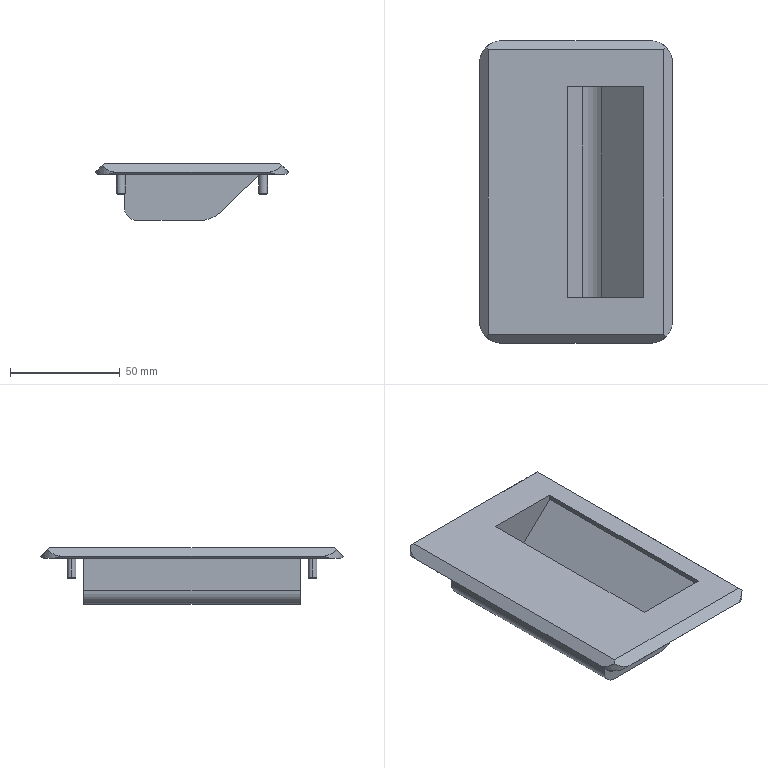Part | SolidWorks | features BaseBody 1 | 1 solid | 48 faces | box 88 x 138 x 26 mm | volume 105651 mm3 | plane 25 | cylinder 15 | cone 8 | commonest cylinder face diameters 4 x8 20 x4 24.8 x2 12.4 x1
STEP:
#1=CARTESIAN_POINT('',(34.5,55.,-8.621));
#2=VERTEX_POINT('',#1);
#3=CARTESIAN_POINT('',(30.5,55.,-8.621));
#4=VERTEX_POINT('',#3);
#5=CARTESIAN_POINT('',(32.5,55.,-8.621));
#6=DIRECTION('',(0.,0.,1.));
#7=DIRECTION('',(1.,0.,0.));
#8=AXIS2_PLACEMENT_3D('',#5,#6,#7);
#9=CIRCLE('',#8,2.);
#10=EDGE_CURVE('',#2,#4,#9,.T.);
#11=ORIENTED_EDGE('',*,*,#10,.T.);
#12=CARTESIAN_POINT('',(30.5,55.,0.));
#13=VERTEX_POINT('',#12);
#14=CARTESIAN_POINT('',(30.5,55.,-4.311));
#15=DIRECTION('',(0.,0.,1.));
#16=VECTOR('',#15,1000.);
#17=LINE('',#14,#16);
#18=EDGE_CURVE('',#4,#13,#17,.T.);
#19=ORIENTED_EDGE('',*,*,#18,.T.);
#20=CARTESIAN_POINT('',(34.5,55.,0.));
#21=VERTEX_POINT('',#20);
#22=CARTESIAN_POINT('',(32.5,55.,0.));
#23=DIRECTION('',(0.,0.,-1.));
#24=DIRECTION('',(1.,0.,0.));
#25=AXIS2_PLACEMENT_3D('',#22,#23,#24);
#26=CIRCLE('',#25,2.);
#27=EDGE_CURVE('',#13,#21,#26,.T.);
#28=ORIENTED_EDGE('',*,*,#27,.T.);
#29=CARTESIAN_POINT('',(34.5,55.,-4.311));
#30=DIRECTION('',(0.,0.,1.));
#31=VECTOR('',#30,1000.);
#32=LINE('',#29,#31);
#33=EDGE_CURVE('',#2,#21,#32,.T.);
#34=ORIENTED_EDGE('',*,*,#33,.F.);
#35=EDGE_LOOP('',(#11,#19,#28,#34));
#36=FACE_OUTER_BOUND('',#35,.T.);
#37=CARTESIAN_POINT('',(32.5,55.,-4.311));
#38=DIRECTION('',(0.,0.,1.));
#39=DIRECTION('',(1.,0.,0.));
#40=AXIS2_PLACEMENT_3D('',#37,#38,#39);
#41=CYLINDRICAL_SURFACE('',#40,2.);
#42=ADVANCED_FACE('',(#36),#41,.T.);
#43=CARTESIAN_POINT('',(34.5,-55.,-8.621));
#44=VERTEX_POINT('',#43);
#45=CARTESIAN_POINT('',(30.5,-55.,-8.621));
#46=VERTEX_POINT('',#45);
#47=CARTESIAN_POINT('',(32.5,-55.,-8.621));
#48=DIRECTION('',(0.,0.,1.));
#49=DIRECTION('',(1.,0.,0.));
#50=AXIS2_PLACEMENT_3D('',#47,#48,#49);
#51=CIRCLE('',#50,2.);
#52=EDGE_CURVE('',#44,#46,#51,.T.);
#53=ORIENTED_EDGE('',*,*,#52,.T.);
#54=CARTESIAN_POINT('',(30.5,-55.,0.));
#55=VERTEX_POINT('',#54);
#56=CARTESIAN_POINT('',(30.5,-55.,-4.311));
#57=DIRECTION('',(0.,0.,1.));
#58=VECTOR('',#57,1000.);
#59=LINE('',#56,#58);
#60=EDGE_CURVE('',#46,#55,#59,.T.);
#61=ORIENTED_EDGE('',*,*,#60,.T.);
#62=CARTESIAN_POINT('',(34.5,-55.,0.));
#63=VERTEX_POINT('',#62);
#64=CARTESIAN_POINT('',(32.5,-55.,0.));
#65=DIRECTION('',(0.,0.,-1.));
#66=DIRECTION('',(1.,0.,0.));
#67=AXIS2_PLACEMENT_3D('',#64,#65,#66);
#68=CIRCLE('',#67,2.);
#69=EDGE_CURVE('',#55,#63,#68,.T.);
#70=ORIENTED_EDGE('',*,*,#69,.T.);
#71=CARTESIAN_POINT('',(34.5,-55.,-4.311));
#72=DIRECTION('',(0.,0.,1.));
#73=VECTOR('',#72,1000.);
#74=LINE('',#71,#73);
#75=EDGE_CURVE('',#44,#63,#74,.T.);
#76=ORIENTED_EDGE('',*,*,#75,.F.);
#77=EDGE_LOOP('',(#53,#61,#70,#76));
#78=FACE_OUTER_BOUND('',#77,.T.);
#79=CARTESIAN_POINT('',(32.5,-55.,-4.311));
#80=DIRECTION('',(0.,0.,1.));
#81=DIRECTION('',(1.,0.,0.));
#82=AXIS2_PLACEMENT_3D('',#79,#80,#81);
#83=CYLINDRICAL_SURFACE('',#82,2.);
#84=ADVANCED_FACE('',(#78),#83,.T.);
#85=CARTESIAN_POINT('',(-30.5,-55.,-8.621));
#86=VERTEX_POINT('',#85);
#87=CARTESIAN_POINT('',(-34.5,-55.,-8.621));
#88=VERTEX_POINT('',#87);
#89=CARTESIAN_POINT('',(-32.5,-55.,-8.621));
#90=DIRECTION('',(0.,0.,1.));
#91=DIRECTION('',(1.,0.,0.));
#92=AXIS2_PLACEMENT_3D('',#89,#90,#91);
#93=CIRCLE('',#92,2.);
#94=EDGE_CURVE('',#86,#88,#93,.T.);
#95=ORIENTED_EDGE('',*,*,#94,.T.);
#96=CARTESIAN_POINT('',(-34.5,-55.,0.));
#97=VERTEX_POINT('',#96);
#98=CARTESIAN_POINT('',(-34.5,-55.,-4.311));
#99=DIRECTION('',(0.,0.,1.));
#100=VECTOR('',#99,1000.);
#101=LINE('',#98,#100);
#102=EDGE_CURVE('',#88,#97,#101,.T.);
#103=ORIENTED_EDGE('',*,*,#102,.T.);
#104=CARTESIAN_POINT('',(-30.5,-55.,0.));
#105=VERTEX_POINT('',#104);
#106=CARTESIAN_POINT('',(-32.5,-55.,0.));
#107=DIRECTION('',(0.,0.,-1.));
#108=DIRECTION('',(1.,0.,0.));
#109=AXIS2_PLACEMENT_3D('',#106,#107,#108);
#110=CIRCLE('',#109,2.);
#111=EDGE_CURVE('',#97,#105,#110,.T.);
#112=ORIENTED_EDGE('',*,*,#111,.T.);
#113=CARTESIAN_POINT('',(-30.5,-55.,-4.311));
#114=DIRECTION('',(0.,0.,1.));
#115=VECTOR('',#114,1000.);
#116=LINE('',#113,#115);
#117=EDGE_CURVE('',#86,#105,#116,.T.);
#118=ORIENTED_EDGE('',*,*,#117,.F.);
#119=EDGE_LOOP('',(#95,#103,#112,#118));
#120=FACE_OUTER_BOUND('',#119,.T.);
#121=CARTESIAN_POINT('',(-32.5,-55.,-4.311));
#122=DIRECTION('',(0.,0.,1.));
#123=DIRECTION('',(1.,0.,0.));
#124=AXIS2_PLACEMENT_3D('',#121,#122,#123);
#125=CYLINDRICAL_SURFACE('',#124,2.);
#126=ADVANCED_FACE('',(#120),#125,.T.);
#127=CARTESIAN_POINT('',(-30.5,55.,-8.621));
#128=VERTEX_POINT('',#127);
#129=CARTESIAN_POINT('',(-34.5,55.,-8.621));
#130=VERTEX_POINT('',#129);
#131=CARTESIAN_POINT('',(-32.5,55.,-8.621));
#132=DIRECTION('',(0.,0.,1.));
#133=DIRECTION('',(1.,0.,0.));
#134=AXIS2_PLACEMENT_3D('',#131,#132,#133);
#135=CIRCLE('',#134,2.);
#136=EDGE_CURVE('',#128,#130,#135,.T.);
#137=ORIENTED_EDGE('',*,*,#136,.T.);
#138=CARTESIAN_POINT('',(-34.5,55.,0.));
#139=VERTEX_POINT('',#138);
#140=CARTESIAN_POINT('',(-34.5,55.,-4.311));
#141=DIRECTION('',(0.,0.,1.));
#142=VECTOR('',#141,1000.);
#143=LINE('',#140,#142);
#144=EDGE_CURVE('',#130,#139,#143,.T.);
#145=ORIENTED_EDGE('',*,*,#144,.T.);
#146=CARTESIAN_POINT('',(-30.5,55.,0.));
#147=VERTEX_POINT('',#146);
#148=CARTESIAN_POINT('',(-32.5,55.,0.));
#149=DIRECTION('',(0.,0.,-1.));
#150=DIRECTION('',(1.,0.,0.));
#151=AXIS2_PLACEMENT_3D('',#148,#149,#150);
#152=CIRCLE('',#151,2.);
#153=EDGE_CURVE('',#139,#147,#152,.T.);
#154=ORIENTED_EDGE('',*,*,#153,.T.);
#155=CARTESIAN_POINT('',(-30.5,55.,-4.311));
#156=DIRECTION('',(0.,0.,1.));
#157=VECTOR('',#156,1000.);
#158=LINE('',#155,#157);
#159=EDGE_CURVE('',#128,#147,#158,.T.);
#160=ORIENTED_EDGE('',*,*,#159,.F.);
#161=EDGE_LOOP('',(#137,#145,#154,#160));
#162=FACE_OUTER_BOUND('',#161,.T.);
#163=CARTESIAN_POINT('',(-32.5,55.,-4.311));
#164=DIRECTION('',(0.,0.,1.));
#165=DIRECTION('',(1.,0.,0.));
#166=AXIS2_PLACEMENT_3D('',#163,#164,#165);
#167=CYLINDRICAL_SURFACE('',#166,2.);
#168=ADVANCED_FACE('',(#162),#167,.T.);
#169=CARTESIAN_POINT('',(34.121,55.,-9.));
#170=VERTEX_POINT('',#169);
#171=CARTESIAN_POINT('',(30.879,55.,-9.));
#172=VERTEX_POINT('',#171);
#173=CARTESIAN_POINT('',(32.5,55.,-9.));
#174=DIRECTION('',(0.,0.,1.));
#175=DIRECTION('',(1.,0.,0.));
#176=AXIS2_PLACEMENT_3D('',#173,#174,#175);
#177=CIRCLE('',#176,1.621);
#178=EDGE_CURVE('',#170,#172,#177,.T.);
#179=ORIENTED_EDGE('',*,*,#178,.T.);
#180=CARTESIAN_POINT('',(30.5,55.,-8.621));
#181=DIRECTION('',(-0.7071,0.,0.7071));
#182=VECTOR('',#181,1000.);
#183=LINE('',#180,#182);
#184=EDGE_CURVE('',#172,#4,#183,.T.);
#185=ORIENTED_EDGE('',*,*,#184,.T.);
#186=ORIENTED_EDGE('',*,*,#10,.F.);
#187=CARTESIAN_POINT('',(34.5,55.,-8.621));
#188=DIRECTION('',(0.7071,0.,0.7071));
#189=VECTOR('',#188,1000.);
#190=LINE('',#187,#189);
#191=EDGE_CURVE('',#170,#2,#190,.T.);
#192=ORIENTED_EDGE('',*,*,#191,.F.);
#193=EDGE_LOOP('',(#179,#185,#186,#192));
#194=FACE_OUTER_BOUND('',#193,.T.);
#195=CARTESIAN_POINT('',(32.5,55.,-8.621));
#196=DIRECTION('',(0.,0.,1.));
#197=DIRECTION('',(1.,0.,0.));
#198=AXIS2_PLACEMENT_3D('',#195,#196,#197);
#199=CONICAL_SURFACE('',#198,2.,0.7854);
#200=ADVANCED_FACE('',(#194),#199,.T.);
#201=CARTESIAN_POINT('',(34.121,-55.,-9.));
#202=VERTEX_POINT('',#201);
#203=CARTESIAN_POINT('',(30.879,-55.,-9.));
#204=VERTEX_POINT('',#203);
#205=CARTESIAN_POINT('',(32.5,-55.,-9.));
#206=DIRECTION('',(0.,0.,1.));
#207=DIRECTION('',(1.,0.,0.));
#208=AXIS2_PLACEMENT_3D('',#205,#206,#207);
#209=CIRCLE('',#208,1.621);
#210=EDGE_CURVE('',#202,#204,#209,.T.);
#211=ORIENTED_EDGE('',*,*,#210,.T.);
#212=CARTESIAN_POINT('',(30.5,-55.,-8.621));
#213=DIRECTION('',(-0.7071,0.,0.7071));
#214=VECTOR('',#213,1000.);
#215=LINE('',#212,#214);
#216=EDGE_CURVE('',#204,#46,#215,.T.);
#217=ORIENTED_EDGE('',*,*,#216,.T.);
#218=ORIENTED_EDGE('',*,*,#52,.F.);
#219=CARTESIAN_POINT('',(34.5,-55.,-8.621));
#220=DIRECTION('',(0.7071,0.,0.7071));
#221=VECTOR('',#220,1000.);
#222=LINE('',#219,#221);
#223=EDGE_CURVE('',#202,#44,#222,.T.);
#224=ORIENTED_EDGE('',*,*,#223,.F.);
#225=EDGE_LOOP('',(#211,#217,#218,#224));
#226=FACE_OUTER_BOUND('',#225,.T.);
#227=CARTESIAN_POINT('',(32.5,-55.,-8.621));
#228=DIRECTION('',(0.,0.,1.));
#229=DIRECTION('',(1.,0.,0.));
#230=AXIS2_PLACEMENT_3D('',#227,#228,#229);
#231=CONICAL_SURFACE('',#230,2.,0.7854);
#232=ADVANCED_FACE('',(#226),#231,.T.);
#233=CARTESIAN_POINT('',(-30.879,-55.,-9.));
#234=VERTEX_POINT('',#233);
#235=CARTESIAN_POINT('',(-34.121,-55.,-9.));
#236=VERTEX_POINT('',#235);
#237=CARTESIAN_POINT('',(-32.5,-55.,-9.));
#238=DIRECTION('',(0.,0.,1.));
#239=DIRECTION('',(1.,0.,0.));
#240=AXIS2_PLACEMENT_3D('',#237,#238,#239);
#241=CIRCLE('',#240,1.621);
#242=EDGE_CURVE('',#234,#236,#241,.T.);
#243=ORIENTED_EDGE('',*,*,#242,.T.);
#244=CARTESIAN_POINT('',(-34.5,-55.,-8.621));
#245=DIRECTION('',(-0.7071,0.,0.7071));
#246=VECTOR('',#245,1000.);
#247=LINE('',#244,#246);
#248=EDGE_CURVE('',#236,#88,#247,.T.);
#249=ORIENTED_EDGE('',*,*,#248,.T.);
#250=ORIENTED_EDGE('',*,*,#94,.F.);
#251=CARTESIAN_POINT('',(-30.5,-55.,-8.621));
#252=DIRECTION('',(0.7071,0.,0.7071));
#253=VECTOR('',#252,1000.);
#254=LINE('',#251,#253);
#255=EDGE_CURVE('',#234,#86,#254,.T.);
#256=ORIENTED_EDGE('',*,*,#255,.F.);
#257=EDGE_LOOP('',(#243,#249,#250,#256));
#258=FACE_OUTER_BOUND('',#257,.T.);
#259=CARTESIAN_POINT('',(-32.5,-55.,-8.621));
#260=DIRECTION('',(0.,0.,1.));
#261=DIRECTION('',(1.,0.,0.));
#262=AXIS2_PLACEMENT_3D('',#259,#260,#261);
#263=CONICAL_SURFACE('',#262,2.,0.7854);
#264=ADVANCED_FACE('',(#258),#263,.T.);
#265=CARTESIAN_POINT('',(-30.879,55.,-9.));
#266=VERTEX_POINT('',#265);
#267=CARTESIAN_POINT('',(-34.121,55.,-9.));
#268=VERTEX_POINT('',#267);
#269=CARTESIAN_POINT('',(-32.5,55.,-9.));
#270=DIRECTION('',(0.,0.,1.));
#271=DIRECTION('',(1.,0.,0.));
#272=AXIS2_PLACEMENT_3D('',#269,#270,#271);
#273=CIRCLE('',#272,1.621);
#274=EDGE_CURVE('',#266,#268,#273,.T.);
#275=ORIENTED_EDGE('',*,*,#274,.T.);
#276=CARTESIAN_POINT('',(-34.5,55.,-8.621));
#277=DIRECTION('',(-0.7071,0.,0.7071));
#278=VECTOR('',#277,1000.);
#279=LINE('',#276,#278);
#280=EDGE_CURVE('',#268,#130,#279,.T.);
#281=ORIENTED_EDGE('',*,*,#280,.T.);
#282=ORIENTED_EDGE('',*,*,#136,.F.);
#283=CARTESIAN_POINT('',(-30.5,55.,-8.621));
#284=DIRECTION('',(0.7071,0.,0.7071));
#285=VECTOR('',#284,1000.);
#286=LINE('',#283,#285);
#287=EDGE_CURVE('',#266,#128,#286,.T.);
#288=ORIENTED_EDGE('',*,*,#287,.F.);
#289=EDGE_LOOP('',(#275,#281,#282,#288));
#290=FACE_OUTER_BOUND('',#289,.T.);
#291=CARTESIAN_POINT('',(-32.5,55.,-8.621));
#292=DIRECTION('',(0.,0.,1.));
#293=DIRECTION('',(1.,0.,0.));
#294=AXIS2_PLACEMENT_3D('',#291,#292,#293);
#295=CONICAL_SURFACE('',#294,2.,0.7854);
#296=ADVANCED_FACE('',(#290),#295,.T.);
#297=ORIENTED_EDGE('',*,*,#274,.F.);
#298=CARTESIAN_POINT('',(-32.5,55.,-9.));
#299=DIRECTION('',(0.,0.,1.));
#300=DIRECTION('',(1.,0.,0.));
#301=AXIS2_PLACEMENT_3D('',#298,#299,#300);
#302=CIRCLE('',#301,1.621);
#303=EDGE_CURVE('',#268,#266,#302,.T.);
#304=ORIENTED_EDGE('',*,*,#303,.F.);
#305=EDGE_LOOP('',(#297,#304));
#306=FACE_OUTER_BOUND('',#305,.T.);
#307=CARTESIAN_POINT('',(-31.69,55.,-9.));
#308=DIRECTION('',(0.,0.,-1.));
#309=DIRECTION('',(0.,-1.,0.));
#310=AXIS2_PLACEMENT_3D('',#307,#308,#309);
#311=PLANE('',#310);
#312=ADVANCED_FACE('',(#306),#311,.T.);
#313=ORIENTED_EDGE('',*,*,#242,.F.);
#314=CARTESIAN_POINT('',(-32.5,-55.,-9.));
#315=DIRECTION('',(0.,0.,1.));
#316=DIRECTION('',(1.,0.,0.));
#317=AXIS2_PLACEMENT_3D('',#314,#315,#316);
#318=CIRCLE('',#317,1.621);
#319=EDGE_CURVE('',#236,#234,#318,.T.);
#320=ORIENTED_EDGE('',*,*,#319,.F.);
#321=EDGE_LOOP('',(#313,#320));
#322=FACE_OUTER_BOUND('',#321,.T.);
#323=CARTESIAN_POINT('',(-31.69,-55.,-9.));
#324=DIRECTION('',(0.,0.,-1.));
#325=DIRECTION('',(0.,-1.,0.));
#326=AXIS2_PLACEMENT_3D('',#323,#324,#325);
#327=PLANE('',#326);
#328=ADVANCED_FACE('',(#322),#327,.T.);
#329=ORIENTED_EDGE('',*,*,#210,.F.);
#330=CARTESIAN_POINT('',(32.5,-55.,-9.));
#331=DIRECTION('',(0.,0.,1.));
#332=DIRECTION('',(1.,0.,0.));
#333=AXIS2_PLACEMENT_3D('',#330,#331,#332);
#334=CIRCLE('',#333,1.621);
#335=EDGE_CURVE('',#204,#202,#334,.T.);
#336=ORIENTED_EDGE('',*,*,#335,.F.);
#337=EDGE_LOOP('',(#329,#336));
#338=FACE_OUTER_BOUND('',#337,.T.);
#339=CARTESIAN_POINT('',(33.31,-55.,-9.));
#340=DIRECTION('',(0.,0.,-1.));
#341=DIRECTION('',(0.,-1.,0.));
#342=AXIS2_PLACEMENT_3D('',#339,#340,#341);
#343=PLANE('',#342);
#344=ADVANCED_FACE('',(#338),#343,.T.);
#345=ORIENTED_EDGE('',*,*,#178,.F.);
#346=CARTESIAN_POINT('',(32.5,55.,-9.));
#347=DIRECTION('',(0.,0.,1.));
#348=DIRECTION('',(1.,0.,0.));
#349=AXIS2_PLACEMENT_3D('',#346,#347,#348);
#350=CIRCLE('',#349,1.621);
#351=EDGE_CURVE('',#172,#170,#350,.T.);
#352=ORIENTED_EDGE('',*,*,#351,.F.);
#353=EDGE_LOOP('',(#345,#352));
#354=FACE_OUTER_BOUND('',#353,.T.);
#355=CARTESIAN_POINT('',(33.31,55.,-9.));
#356=DIRECTION('',(0.,0.,-1.));
#357=DIRECTION('',(0.,-1.,0.));
#358=AXIS2_PLACEMENT_3D('',#355,#356,#357);
#359=PLANE('',#358);
#360=ADVANCED_FACE('',(#354),#359,.T.);
#361=CARTESIAN_POINT('',(12.445,49.5,-17.597));
#362=VERTEX_POINT('',#361);
#363=CARTESIAN_POINT('',(3.912,49.5,-21.));
#364=VERTEX_POINT('',#363);
#365=CARTESIAN_POINT('',(3.912,49.5,-8.6));
#366=DIRECTION('',(0.,1.,0.));
#367=DIRECTION('',(0.,0.,1.));
#368=AXIS2_PLACEMENT_3D('',#365,#366,#367);
#369=CIRCLE('',#368,12.4);
#370=EDGE_CURVE('',#362,#364,#369,.T.);
#371=ORIENTED_EDGE('',*,*,#370,.F.);
#372=CARTESIAN_POINT('',(12.445,-49.5,-17.597));
#373=VERTEX_POINT('',#372);
#374=CARTESIAN_POINT('',(12.445,49.5,-17.597));
#375=DIRECTION('',(0.,1.,0.));
#376=VECTOR('',#375,1000.);
#377=LINE('',#374,#376);
#378=EDGE_CURVE('',#373,#362,#377,.T.);
#379=ORIENTED_EDGE('',*,*,#378,.F.);
#380=CARTESIAN_POINT('',(3.912,-49.5,-21.));
#381=VERTEX_POINT('',#380);
#382=CARTESIAN_POINT('',(3.912,-49.5,-8.6));
#383=DIRECTION('',(0.,1.,0.));
#384=DIRECTION('',(0.,0.,1.));
#385=AXIS2_PLACEMENT_3D('',#382,#383,#384);
#386=CIRCLE('',#385,12.4);
#387=EDGE_CURVE('',#373,#381,#386,.T.);
#388=ORIENTED_EDGE('',*,*,#387,.T.);
#389=CARTESIAN_POINT('',(3.912,49.5,-21.));
#390=DIRECTION('',(0.,-1.,0.));
#391=VECTOR('',#390,1000.);
#392=LINE('',#389,#391);
#393=EDGE_CURVE('',#364,#381,#392,.T.);
#394=ORIENTED_EDGE('',*,*,#393,.F.);
#395=EDGE_LOOP('',(#371,#379,#388,#394));
#396=FACE_OUTER_BOUND('',#395,.T.);
#397=CARTESIAN_POINT('',(3.912,49.5,-8.6));
#398=DIRECTION('',(0.,1.,0.));
#399=DIRECTION('',(0.,0.,1.));
#400=AXIS2_PLACEMENT_3D('',#397,#398,#399);
#401=CYLINDRICAL_SURFACE('',#400,12.4);
#402=ADVANCED_FACE('',(#396),#401,.T.);
#403=CARTESIAN_POINT('',(-24.8,49.5,-21.));
#404=VERTEX_POINT('',#403);
#405=CARTESIAN_POINT('',(0.,49.5,-21.));
#406=DIRECTION('',(-1.,0.,0.));
#407=VECTOR('',#406,1000.);
#408=LINE('',#405,#407);
#409=EDGE_CURVE('',#364,#404,#408,.T.);
#410=ORIENTED_EDGE('',*,*,#409,.F.);
#411=ORIENTED_EDGE('',*,*,#393,.T.);
#412=CARTESIAN_POINT('',(-24.8,-49.5,-21.));
#413=VERTEX_POINT('',#412);
#414=CARTESIAN_POINT('',(0.,-49.5,-21.));
#415=DIRECTION('',(-1.,0.,0.));
#416=VECTOR('',#415,1000.);
#417=LINE('',#414,#416);
#418=EDGE_CURVE('',#381,#413,#417,.T.);
#419=ORIENTED_EDGE('',*,*,#418,.T.);
#420=CARTESIAN_POINT('',(-24.8,49.5,-21.));
#421=DIRECTION('',(0.,-1.,0.));
#422=VECTOR('',#421,1000.);
#423=LINE('',#420,#422);
#424=EDGE_CURVE('',#404,#413,#423,.T.);
#425=ORIENTED_EDGE('',*,*,#424,.F.);
#426=EDGE_LOOP('',(#410,#411,#419,#425));
#427=FACE_OUTER_BOUND('',#426,.T.);
#428=CARTESIAN_POINT('',(3.912,49.5,-21.));
#429=DIRECTION('',(0.,0.,-1.));
#430=DIRECTION('',(0.,-1.,0.));
#431=AXIS2_PLACEMENT_3D('',#428,#429,#430);
#432=PLANE('',#431);
#433=ADVANCED_FACE('',(#427),#432,.T.);
#434=CARTESIAN_POINT('',(-31.,49.5,-14.8));
#435=VERTEX_POINT('',#434);
#436=CARTESIAN_POINT('',(-24.8,49.5,-14.8));
#437=DIRECTION('',(0.,1.,0.));
#438=DIRECTION('',(0.,0.,1.));
#439=AXIS2_PLACEMENT_3D('',#436,#437,#438);
#440=CIRCLE('',#439,6.2);
#441=EDGE_CURVE('',#404,#435,#440,.T.);
#442=ORIENTED_EDGE('',*,*,#441,.F.);
#443=ORIENTED_EDGE('',*,*,#424,.T.);
#444=CARTESIAN_POINT('',(-31.,-49.5,-14.8));
#445=VERTEX_POINT('',#444);
#446=CARTESIAN_POINT('',(-24.8,-49.5,-14.8));
#447=DIRECTION('',(0.,1.,0.));
#448=DIRECTION('',(0.,0.,1.));
#449=AXIS2_PLACEMENT_3D('',#446,#447,#448);
#450=CIRCLE('',#449,6.2);
#451=EDGE_CURVE('',#413,#445,#450,.T.);
#452=ORIENTED_EDGE('',*,*,#451,.T.);
#453=CARTESIAN_POINT('',(-31.,49.5,-14.8));
#454=DIRECTION('',(0.,-1.,0.));
#455=VECTOR('',#454,1000.);
#456=LINE('',#453,#455);
#457=EDGE_CURVE('',#435,#445,#456,.T.);
#458=ORIENTED_EDGE('',*,*,#457,.F.);
#459=EDGE_LOOP('',(#442,#443,#452,#458));
#460=FACE_OUTER_BOUND('',#459,.T.);
#461=CARTESIAN_POINT('',(-24.8,49.5,-14.8));
#462=DIRECTION('',(0.,1.,0.));
#463=DIRECTION('',(0.,0.,1.));
#464=AXIS2_PLACEMENT_3D('',#461,#462,#463);
#465=CYLINDRICAL_SURFACE('',#464,6.2);
#466=ADVANCED_FACE('',(#460),#465,.T.);
#467=ORIENTED_EDGE('',*,*,#409,.T.);
#468=ORIENTED_EDGE('',*,*,#441,.T.);
#469=CARTESIAN_POINT('',(-31.,49.5,0.));
#470=VERTEX_POINT('',#469);
#471=CARTESIAN_POINT('',(-31.,49.5,-14.8));
#472=DIRECTION('',(0.,0.,-1.));
#473=VECTOR('',#472,1000.);
#474=LINE('',#471,#473);
#475=EDGE_CURVE('',#470,#435,#474,.T.);
#476=ORIENTED_EDGE('',*,*,#475,.F.);
#477=CARTESIAN_POINT('',(31.,49.5,0.));
#478=VERTEX_POINT('',#477);
#479=CARTESIAN_POINT('',(0.,49.5,0.));
#480=DIRECTION('',(1.,0.,0.));
#481=VECTOR('',#480,1000.);
#482=LINE('',#479,#481);
#483=EDGE_CURVE('',#470,#478,#482,.T.);
#484=ORIENTED_EDGE('',*,*,#483,.T.);
#485=CARTESIAN_POINT('',(31.,49.5,0.));
#486=DIRECTION('',(0.7256,0.,0.6881));
#487=VECTOR('',#486,1000.);
#488=LINE('',#485,#487);
#489=EDGE_CURVE('',#362,#478,#488,.T.);
#490=ORIENTED_EDGE('',*,*,#489,.F.);
#491=ORIENTED_EDGE('',*,*,#370,.T.);
#492=EDGE_LOOP('',(#467,#468,#476,#484,#490,#491));
#493=FACE_OUTER_BOUND('',#492,.T.);
#494=CARTESIAN_POINT('',(0.,49.5,0.));
#495=DIRECTION('',(0.,1.,0.));
#496=DIRECTION('',(1.,0.,0.));
#497=AXIS2_PLACEMENT_3D('',#494,#495,#496);
#498=PLANE('',#497);
#499=ADVANCED_FACE('',(#493),#498,.T.);
#500=ORIENTED_EDGE('',*,*,#489,.T.);
#501=CARTESIAN_POINT('',(31.,-49.5,0.));
#502=VERTEX_POINT('',#501);
#503=CARTESIAN_POINT('',(31.,0.,0.));
#504=DIRECTION('',(0.,-1.,0.));
#505=VECTOR('',#504,1000.);
#506=LINE('',#503,#505);
#507=EDGE_CURVE('',#478,#502,#506,.T.);
#508=ORIENTED_EDGE('',*,*,#507,.T.);
#509=CARTESIAN_POINT('',(31.,-49.5,0.));
#510=DIRECTION('',(-0.7256,0.,-0.6881));
#511=VECTOR('',#510,1000.);
#512=LINE('',#509,#511);
#513=EDGE_CURVE('',#502,#373,#512,.T.);
#514=ORIENTED_EDGE('',*,*,#513,.T.);
#515=ORIENTED_EDGE('',*,*,#378,.T.);
#516=EDGE_LOOP('',(#500,#508,#514,#515));
#517=FACE_OUTER_BOUND('',#516,.T.);
#518=CARTESIAN_POINT('',(31.,49.5,0.));
#519=DIRECTION('',(0.6881,0.,-0.7256));
#520=DIRECTION('',(0.,-1.,0.));
#521=AXIS2_PLACEMENT_3D('',#518,#519,#520);
#522=PLANE('',#521);
#523=ADVANCED_FACE('',(#517),#522,.T.);
#524=CARTESIAN_POINT('',(-31.,-49.5,0.));
#525=VERTEX_POINT('',#524);
#526=CARTESIAN_POINT('',(-31.,-49.5,-14.8));
#527=DIRECTION('',(0.,0.,1.));
#528=VECTOR('',#527,1000.);
#529=LINE('',#526,#528);
#530=EDGE_CURVE('',#445,#525,#529,.T.);
#531=ORIENTED_EDGE('',*,*,#530,.F.);
#532=ORIENTED_EDGE('',*,*,#451,.F.);
#533=ORIENTED_EDGE('',*,*,#418,.F.);
#534=ORIENTED_EDGE('',*,*,#387,.F.);
#535=ORIENTED_EDGE('',*,*,#513,.F.);
#536=CARTESIAN_POINT('',(0.,-49.5,0.));
#537=DIRECTION('',(-1.,0.,0.));
#538=VECTOR('',#537,1000.);
#539=LINE('',#536,#538);
#540=EDGE_CURVE('',#502,#525,#539,.T.);
#541=ORIENTED_EDGE('',*,*,#540,.T.);
#542=EDGE_LOOP('',(#531,#532,#533,#534,#535,#541));
#543=FACE_OUTER_BOUND('',#542,.T.);
#544=CARTESIAN_POINT('',(0.,-49.5,0.));
#545=DIRECTION('',(0.,1.,0.));
#546=DIRECTION('',(1.,0.,0.));
#547=AXIS2_PLACEMENT_3D('',#544,#545,#546);
#548=PLANE('',#547);
#549=ADVANCED_FACE('',(#543),#548,.F.);
#550=ORIENTED_EDGE('',*,*,#475,.T.);
#551=ORIENTED_EDGE('',*,*,#457,.T.);
#552=ORIENTED_EDGE('',*,*,#530,.T.);
#553=CARTESIAN_POINT('',(-31.,0.,0.));
#554=DIRECTION('',(0.,1.,0.));
#555=VECTOR('',#554,1000.);
#556=LINE('',#553,#555);
#557=EDGE_CURVE('',#525,#470,#556,.T.);
#558=ORIENTED_EDGE('',*,*,#557,.T.);
#559=EDGE_LOOP('',(#550,#551,#552,#558));
#560=FACE_OUTER_BOUND('',#559,.T.);
#561=CARTESIAN_POINT('',(-31.,49.5,-14.8));
#562=DIRECTION('',(-1.,0.,0.));
#563=DIRECTION('',(0.,1.,0.));
#564=AXIS2_PLACEMENT_3D('',#561,#562,#563);
#565=PLANE('',#564);
#566=ADVANCED_FACE('',(#560),#565,.T.);
#567=CARTESIAN_POINT('',(-32.5,55.,0.));
#568=DIRECTION('',(0.,0.,-1.));
#569=DIRECTION('',(1.,0.,0.));
#570=AXIS2_PLACEMENT_3D('',#567,#568,#569);
#571=CIRCLE('',#570,2.);
#572=EDGE_CURVE('',#147,#139,#571,.T.);
#573=ORIENTED_EDGE('',*,*,#572,.F.);
#574=ORIENTED_EDGE('',*,*,#153,.F.);
#575=EDGE_LOOP('',(#573,#574));
#576=FACE_BOUND('',#575,.T.);
#577=CARTESIAN_POINT('',(-32.5,-55.,0.));
#578=DIRECTION('',(0.,0.,-1.));
#579=DIRECTION('',(1.,0.,0.));
#580=AXIS2_PLACEMENT_3D('',#577,#578,#579);
#581=CIRCLE('',#580,2.);
#582=EDGE_CURVE('',#105,#97,#581,.T.);
#583=ORIENTED_EDGE('',*,*,#582,.F.);
#584=ORIENTED_EDGE('',*,*,#111,.F.);
#585=EDGE_LOOP('',(#583,#584));
#586=FACE_BOUND('',#585,.T.);
#587=CARTESIAN_POINT('',(32.5,-55.,0.));
#588=DIRECTION('',(0.,0.,-1.));
#589=DIRECTION('',(1.,0.,0.));
#590=AXIS2_PLACEMENT_3D('',#587,#588,#589);
#591=CIRCLE('',#590,2.);
#592=EDGE_CURVE('',#63,#55,#591,.T.);
#593=ORIENTED_EDGE('',*,*,#592,.F.);
#594=ORIENTED_EDGE('',*,*,#69,.F.);
#595=EDGE_LOOP('',(#593,#594));
#596=FACE_BOUND('',#595,.T.);
#597=CARTESIAN_POINT('',(32.5,55.,0.));
#598=DIRECTION('',(0.,0.,-1.));
#599=DIRECTION('',(1.,0.,0.));
#600=AXIS2_PLACEMENT_3D('',#597,#598,#599);
#601=CIRCLE('',#600,2.);
#602=EDGE_CURVE('',#21,#13,#601,.T.);
#603=ORIENTED_EDGE('',*,*,#602,.F.);
#604=ORIENTED_EDGE('',*,*,#27,.F.);
#605=EDGE_LOOP('',(#603,#604));
#606=FACE_BOUND('',#605,.T.);
#607=ORIENTED_EDGE('',*,*,#540,.F.);
#608=ORIENTED_EDGE('',*,*,#507,.F.);
#609=ORIENTED_EDGE('',*,*,#483,.F.);
#610=ORIENTED_EDGE('',*,*,#557,.F.);
#611=EDGE_LOOP('',(#607,#608,#609,#610));
#612=FACE_BOUND('',#611,.T.);
#613=CARTESIAN_POINT('',(-38.359,68.,0.));
#614=VERTEX_POINT('',#613);
#615=CARTESIAN_POINT('',(-43.,63.359,0.));
#616=VERTEX_POINT('',#615);
#617=CARTESIAN_POINT('',(-34.,59.,0.));
#618=DIRECTION('',(0.,0.,1.));
#619=DIRECTION('',(-1.,0.,0.));
#620=AXIS2_PLACEMENT_3D('',#617,#618,#619);
#621=CIRCLE('',#620,10.);
#622=EDGE_CURVE('',#614,#616,#621,.T.);
#623=ORIENTED_EDGE('',*,*,#622,.F.);
#624=CARTESIAN_POINT('',(38.359,68.,0.));
#625=VERTEX_POINT('',#624);
#626=CARTESIAN_POINT('',(44.,68.,0.));
#627=DIRECTION('',(1.,0.,0.));
#628=VECTOR('',#627,1000.);
#629=LINE('',#626,#628);
#630=EDGE_CURVE('',#614,#625,#629,.T.);
#631=ORIENTED_EDGE('',*,*,#630,.T.);
#632=CARTESIAN_POINT('',(43.,63.359,0.));
#633=VERTEX_POINT('',#632);
#634=CARTESIAN_POINT('',(34.,59.,0.));
#635=DIRECTION('',(0.,0.,1.));
#636=DIRECTION('',(-1.,0.,0.));
#637=AXIS2_PLACEMENT_3D('',#634,#635,#636);
#638=CIRCLE('',#637,10.);
#639=EDGE_CURVE('',#633,#625,#638,.T.);
#640=ORIENTED_EDGE('',*,*,#639,.F.);
#641=CARTESIAN_POINT('',(43.,-63.359,0.));
#642=VERTEX_POINT('',#641);
#643=CARTESIAN_POINT('',(43.,69.,0.));
#644=DIRECTION('',(0.,-1.,0.));
#645=VECTOR('',#644,1000.);
#646=LINE('',#643,#645);
#647=EDGE_CURVE('',#633,#642,#646,.T.);
#648=ORIENTED_EDGE('',*,*,#647,.T.);
#649=CARTESIAN_POINT('',(38.359,-68.,0.));
#650=VERTEX_POINT('',#649);
#651=CARTESIAN_POINT('',(34.,-59.,0.));
#652=DIRECTION('',(0.,0.,1.));
#653=DIRECTION('',(-1.,0.,0.));
#654=AXIS2_PLACEMENT_3D('',#651,#652,#653);
#655=CIRCLE('',#654,10.);
#656=EDGE_CURVE('',#650,#642,#655,.T.);
#657=ORIENTED_EDGE('',*,*,#656,.F.);
#658=CARTESIAN_POINT('',(-38.359,-68.,0.));
#659=VERTEX_POINT('',#658);
#660=CARTESIAN_POINT('',(44.,-68.,0.));
#661=DIRECTION('',(-1.,0.,0.));
#662=VECTOR('',#661,1000.);
#663=LINE('',#660,#662);
#664=EDGE_CURVE('',#650,#659,#663,.T.);
#665=ORIENTED_EDGE('',*,*,#664,.T.);
#666=CARTESIAN_POINT('',(-43.,-63.359,0.));
#667=VERTEX_POINT('',#666);
#668=CARTESIAN_POINT('',(-34.,-59.,0.));
#669=DIRECTION('',(0.,0.,1.));
#670=DIRECTION('',(-1.,0.,0.));
#671=AXIS2_PLACEMENT_3D('',#668,#669,#670);
#672=CIRCLE('',#671,10.);
#673=EDGE_CURVE('',#667,#659,#672,.T.);
#674=ORIENTED_EDGE('',*,*,#673,.F.);
#675=CARTESIAN_POINT('',(-43.,69.,0.));
#676=DIRECTION('',(0.,1.,0.));
#677=VECTOR('',#676,1000.);
#678=LINE('',#675,#677);
#679=EDGE_CURVE('',#667,#616,#678,.T.);
#680=ORIENTED_EDGE('',*,*,#679,.T.);
#681=EDGE_LOOP('',(#623,#631,#640,#648,#657,#665,#674,#680));
#682=FACE_OUTER_BOUND('',#681,.T.);
#683=CARTESIAN_POINT('',(0.,0.,0.));
#684=DIRECTION('',(0.,0.,1.));
#685=DIRECTION('',(1.,0.,0.));
#686=AXIS2_PLACEMENT_3D('',#683,#684,#685);
#687=PLANE('',#686);
#688=ADVANCED_FACE('',(#576,#586,#596,#606,#612,#682),#687,.F.);
#689=CARTESIAN_POINT('',(31.,-48.,2.756));
#690=VERTEX_POINT('',#689);
#691=CARTESIAN_POINT('',(31.,48.,2.756));
#692=VERTEX_POINT('',#691);
#693=CARTESIAN_POINT('',(31.,48.,2.756));
#694=DIRECTION('',(0.,1.,0.));
#695=VECTOR('',#694,1000.);
#696=LINE('',#693,#695);
#697=EDGE_CURVE('',#690,#692,#696,.T.);
#698=ORIENTED_EDGE('',*,*,#697,.T.);
#699=CARTESIAN_POINT('',(11.648,48.,-15.597));
#700=VERTEX_POINT('',#699);
#701=CARTESIAN_POINT('',(31.,48.,2.756));
#702=DIRECTION('',(-0.7256,0.,-0.6881));
#703=VECTOR('',#702,1000.);
#704=LINE('',#701,#703);
#705=EDGE_CURVE('',#692,#700,#704,.T.);
#706=ORIENTED_EDGE('',*,*,#705,.T.);
#707=CARTESIAN_POINT('',(11.648,-48.,-15.597));
#708=VERTEX_POINT('',#707);
#709=CARTESIAN_POINT('',(11.648,48.,-15.597));
#710=DIRECTION('',(0.,-1.,0.));
#711=VECTOR('',#710,1000.);
#712=LINE('',#709,#711);
#713=EDGE_CURVE('',#700,#708,#712,.T.);
#714=ORIENTED_EDGE('',*,*,#713,.T.);
#715=CARTESIAN_POINT('',(31.,-48.,2.756));
#716=DIRECTION('',(-0.7256,0.,-0.6881));
#717=VECTOR('',#716,1000.);
#718=LINE('',#715,#717);
#719=EDGE_CURVE('',#690,#708,#718,.T.);
#720=ORIENTED_EDGE('',*,*,#719,.F.);
#721=EDGE_LOOP('',(#698,#706,#714,#720));
#722=FACE_OUTER_BOUND('',#721,.T.);
#723=CARTESIAN_POINT('',(31.,48.,2.756));
#724=DIRECTION('',(0.6881,0.,-0.7256));
#725=DIRECTION('',(0.,-1.,0.));
#726=AXIS2_PLACEMENT_3D('',#723,#724,#725);
#727=PLANE('',#726);
#728=ADVANCED_FACE('',(#722),#727,.F.);
#729=ORIENTED_EDGE('',*,*,#713,.F.);
#730=CARTESIAN_POINT('',(3.115,48.,-19.));
#731=VERTEX_POINT('',#730);
#732=CARTESIAN_POINT('',(3.115,48.,-6.6));
#733=DIRECTION('',(0.,1.,0.));
#734=DIRECTION('',(0.,0.,1.));
#735=AXIS2_PLACEMENT_3D('',#732,#733,#734);
#736=CIRCLE('',#735,12.4);
#737=EDGE_CURVE('',#700,#731,#736,.T.);
#738=ORIENTED_EDGE('',*,*,#737,.T.);
#739=CARTESIAN_POINT('',(3.115,-48.,-19.));
#740=VERTEX_POINT('',#739);
#741=CARTESIAN_POINT('',(3.115,48.,-19.));
#742=DIRECTION('',(0.,-1.,0.));
#743=VECTOR('',#742,1000.);
#744=LINE('',#741,#743);
#745=EDGE_CURVE('',#731,#740,#744,.T.);
#746=ORIENTED_EDGE('',*,*,#745,.T.);
#747=CARTESIAN_POINT('',(3.115,-48.,-6.6));
#748=DIRECTION('',(0.,1.,0.));
#749=DIRECTION('',(0.,0.,1.));
#750=AXIS2_PLACEMENT_3D('',#747,#748,#749);
#751=CIRCLE('',#750,12.4);
#752=EDGE_CURVE('',#708,#740,#751,.T.);
#753=ORIENTED_EDGE('',*,*,#752,.F.);
#754=EDGE_LOOP('',(#729,#738,#746,#753));
#755=FACE_OUTER_BOUND('',#754,.T.);
#756=CARTESIAN_POINT('',(3.115,48.,-6.6));
#757=DIRECTION('',(0.,1.,0.));
#758=DIRECTION('',(0.,0.,1.));
#759=AXIS2_PLACEMENT_3D('',#756,#757,#758);
#760=CYLINDRICAL_SURFACE('',#759,12.4);
#761=ADVANCED_FACE('',(#755),#760,.F.);
#762=ORIENTED_EDGE('',*,*,#745,.F.);
#763=CARTESIAN_POINT('',(-4.,48.,-19.));
#764=VERTEX_POINT('',#763);
#765=CARTESIAN_POINT('',(0.,48.,-19.));
#766=DIRECTION('',(-1.,0.,0.));
#767=VECTOR('',#766,1000.);
#768=LINE('',#765,#767);
#769=EDGE_CURVE('',#731,#764,#768,.T.);
#770=ORIENTED_EDGE('',*,*,#769,.T.);
#771=CARTESIAN_POINT('',(-4.,-48.,-19.));
#772=VERTEX_POINT('',#771);
#773=CARTESIAN_POINT('',(-4.,48.,-19.));
#774=DIRECTION('',(0.,-1.,0.));
#775=VECTOR('',#774,1000.);
#776=LINE('',#773,#775);
#777=EDGE_CURVE('',#764,#772,#776,.T.);
#778=ORIENTED_EDGE('',*,*,#777,.T.);
#779=CARTESIAN_POINT('',(0.,-48.,-19.));
#780=DIRECTION('',(-1.,0.,0.));
#781=VECTOR('',#780,1000.);
#782=LINE('',#779,#781);
#783=EDGE_CURVE('',#740,#772,#782,.T.);
#784=ORIENTED_EDGE('',*,*,#783,.F.);
#785=EDGE_LOOP('',(#762,#770,#778,#784));
#786=FACE_OUTER_BOUND('',#785,.T.);
#787=CARTESIAN_POINT('',(3.115,48.,-19.));
#788=DIRECTION('',(0.,0.,-1.));
#789=DIRECTION('',(0.,-1.,0.));
#790=AXIS2_PLACEMENT_3D('',#787,#788,#789);
#791=PLANE('',#790);
#792=ADVANCED_FACE('',(#786),#791,.F.);
#793=CARTESIAN_POINT('',(-44.,-59.,1.));
#794=VERTEX_POINT('',#793);
#795=CARTESIAN_POINT('',(-44.,59.,1.));
#796=VERTEX_POINT('',#795);
#797=CARTESIAN_POINT('',(-44.,69.,1.));
#798=DIRECTION('',(0.,1.,0.));
#799=VECTOR('',#798,1000.);
#800=LINE('',#797,#799);
#801=EDGE_CURVE('',#794,#796,#800,.T.);
#802=ORIENTED_EDGE('',*,*,#801,.T.);
#803=CARTESIAN_POINT('',(-43.,63.359,0.));
#804=CARTESIAN_POINT('',(-43.661,61.994,0.6609));
#805=CARTESIAN_POINT('',(-44.,60.516,1.));
#806=CARTESIAN_POINT('',(-44.,59.,1.));
#807=(BOUNDED_CURVE()B_SPLINE_CURVE(3,(#803,#804,#805,#806),.UNSPECIFIED.,.F.,.T.)B_SPLINE_CURVE_WITH_KNOTS((4,4),(2.691,3.142),.UNSPECIFIED.)CURVE()GEOMETRIC_REPRESENTATION_ITEM()RATIONAL_B_SPLINE_CURVE((1.,0.9831,0.9831,1.))REPRESENTATION_ITEM(''));
#808=EDGE_CURVE('',#616,#796,#807,.T.);
#809=ORIENTED_EDGE('',*,*,#808,.F.);
#810=ORIENTED_EDGE('',*,*,#679,.F.);
#811=CARTESIAN_POINT('',(-44.,-59.,1.));
#812=CARTESIAN_POINT('',(-44.,-60.516,1.));
#813=CARTESIAN_POINT('',(-43.661,-61.994,0.6609));
#814=CARTESIAN_POINT('',(-43.,-63.359,0.));
#815=(BOUNDED_CURVE()B_SPLINE_CURVE(3,(#811,#812,#813,#814),.UNSPECIFIED.,.F.,.T.)B_SPLINE_CURVE_WITH_KNOTS((4,4),(3.142,3.593),.UNSPECIFIED.)CURVE()GEOMETRIC_REPRESENTATION_ITEM()RATIONAL_B_SPLINE_CURVE((1.,0.9831,0.9831,1.))REPRESENTATION_ITEM(''));
#816=EDGE_CURVE('',#794,#667,#815,.T.);
#817=ORIENTED_EDGE('',*,*,#816,.F.);
#818=EDGE_LOOP('',(#802,#809,#810,#817));
#819=FACE_OUTER_BOUND('',#818,.T.);
#820=CARTESIAN_POINT('',(-44.,69.,1.));
#821=DIRECTION('',(0.7071,0.,0.7071));
#822=DIRECTION('',(0.,-1.,0.));
#823=AXIS2_PLACEMENT_3D('',#820,#821,#822);
#824=PLANE('',#823);
#825=ADVANCED_FACE('',(#819),#824,.F.);
#826=CARTESIAN_POINT('',(34.,-69.,1.));
#827=VERTEX_POINT('',#826);
#828=CARTESIAN_POINT('',(-34.,-69.,1.));
#829=VERTEX_POINT('',#828);
#830=CARTESIAN_POINT('',(44.,-69.,1.));
#831=DIRECTION('',(-1.,0.,0.));
#832=VECTOR('',#831,1000.);
#833=LINE('',#830,#832);
#834=EDGE_CURVE('',#827,#829,#833,.T.);
#835=ORIENTED_EDGE('',*,*,#834,.T.);
#836=CARTESIAN_POINT('',(-38.359,-68.,0.));
#837=CARTESIAN_POINT('',(-36.994,-68.661,0.6609));
#838=CARTESIAN_POINT('',(-35.516,-69.,1.));
#839=CARTESIAN_POINT('',(-34.,-69.,1.));
#840=(BOUNDED_CURVE()B_SPLINE_CURVE(3,(#836,#837,#838,#839),.UNSPECIFIED.,.F.,.T.)B_SPLINE_CURVE_WITH_KNOTS((4,4),(2.691,3.142),.UNSPECIFIED.)CURVE()GEOMETRIC_REPRESENTATION_ITEM()RATIONAL_B_SPLINE_CURVE((1.,0.9831,0.9831,1.))REPRESENTATION_ITEM(''));
#841=EDGE_CURVE('',#659,#829,#840,.T.);
#842=ORIENTED_EDGE('',*,*,#841,.F.);
#843=ORIENTED_EDGE('',*,*,#664,.F.);
#844=CARTESIAN_POINT('',(34.,-69.,1.));
#845=CARTESIAN_POINT('',(35.516,-69.,1.));
#846=CARTESIAN_POINT('',(36.994,-68.661,0.6609));
#847=CARTESIAN_POINT('',(38.359,-68.,0.));
#848=(BOUNDED_CURVE()B_SPLINE_CURVE(3,(#844,#845,#846,#847),.UNSPECIFIED.,.F.,.T.)B_SPLINE_CURVE_WITH_KNOTS((4,4),(3.142,3.593),.UNSPECIFIED.)CURVE()GEOMETRIC_REPRESENTATION_ITEM()RATIONAL_B_SPLINE_CURVE((1.,0.9831,0.9831,1.))REPRESENTATION_ITEM(''));
#849=EDGE_CURVE('',#827,#650,#848,.T.);
#850=ORIENTED_EDGE('',*,*,#849,.F.);
#851=EDGE_LOOP('',(#835,#842,#843,#850));
#852=FACE_OUTER_BOUND('',#851,.T.);
#853=CARTESIAN_POINT('',(44.,-68.,0.));
#854=DIRECTION('',(0.,0.7071,0.7071));
#855=DIRECTION('',(1.,0.,0.));
#856=AXIS2_PLACEMENT_3D('',#853,#854,#855);
#857=PLANE('',#856);
#858=ADVANCED_FACE('',(#852),#857,.F.);
#859=CARTESIAN_POINT('',(-41.071,-66.071,3.929));
#860=VERTEX_POINT('',#859);
#861=CARTESIAN_POINT('',(-34.,-69.,1.));
#862=CARTESIAN_POINT('',(-36.688,-69.,1.));
#863=CARTESIAN_POINT('',(-39.171,-67.971,2.029));
#864=CARTESIAN_POINT('',(-41.071,-66.071,3.929));
#865=(BOUNDED_CURVE()B_SPLINE_CURVE(3,(#861,#862,#863,#864),.UNSPECIFIED.,.F.,.T.)B_SPLINE_CURVE_WITH_KNOTS((4,4),(0.,0.7854),.UNSPECIFIED.)CURVE()GEOMETRIC_REPRESENTATION_ITEM()RATIONAL_B_SPLINE_CURVE((1.,0.9493,0.9493,1.))REPRESENTATION_ITEM(''));
#866=EDGE_CURVE('',#829,#860,#865,.T.);
#867=ORIENTED_EDGE('',*,*,#866,.T.);
#868=CARTESIAN_POINT('',(-41.071,-66.071,3.929));
#869=CARTESIAN_POINT('',(-42.971,-64.171,2.029));
#870=CARTESIAN_POINT('',(-44.,-61.688,1.));
#871=CARTESIAN_POINT('',(-44.,-59.,1.));
#872=(BOUNDED_CURVE()B_SPLINE_CURVE(3,(#868,#869,#870,#871),.UNSPECIFIED.,.F.,.T.)B_SPLINE_CURVE_WITH_KNOTS((4,4),(5.498,6.283),.UNSPECIFIED.)CURVE()GEOMETRIC_REPRESENTATION_ITEM()RATIONAL_B_SPLINE_CURVE((1.,0.9493,0.9493,1.))REPRESENTATION_ITEM(''));
#873=EDGE_CURVE('',#860,#794,#872,.T.);
#874=ORIENTED_EDGE('',*,*,#873,.T.);
#875=ORIENTED_EDGE('',*,*,#816,.T.);
#876=ORIENTED_EDGE('',*,*,#673,.T.);
#877=ORIENTED_EDGE('',*,*,#841,.T.);
#878=EDGE_LOOP('',(#867,#874,#875,#876,#877));
#879=FACE_OUTER_BOUND('',#878,.T.);
#880=CARTESIAN_POINT('',(-34.,-59.,0.));
#881=DIRECTION('',(0.,0.,-1.));
#882=DIRECTION('',(-1.,0.,0.));
#883=AXIS2_PLACEMENT_3D('',#880,#881,#882);
#884=CYLINDRICAL_SURFACE('',#883,10.);
#885=ADVANCED_FACE('',(#879),#884,.T.);
#886=ORIENTED_EDGE('',*,*,#647,.F.);
#887=CARTESIAN_POINT('',(44.,59.,1.));
#888=VERTEX_POINT('',#887);
#889=CARTESIAN_POINT('',(44.,59.,1.));
#890=CARTESIAN_POINT('',(44.,60.516,1.));
#891=CARTESIAN_POINT('',(43.661,61.994,0.6609));
#892=CARTESIAN_POINT('',(43.,63.359,0.));
#893=(BOUNDED_CURVE()B_SPLINE_CURVE(3,(#889,#890,#891,#892),.UNSPECIFIED.,.F.,.F.)B_SPLINE_CURVE_WITH_KNOTS((4,4),(3.142,3.593),.UNSPECIFIED.)CURVE()GEOMETRIC_REPRESENTATION_ITEM()RATIONAL_B_SPLINE_CURVE((1.,0.9831,0.9831,1.))REPRESENTATION_ITEM(''));
#894=EDGE_CURVE('',#888,#633,#893,.T.);
#895=ORIENTED_EDGE('',*,*,#894,.F.);
#896=CARTESIAN_POINT('',(44.,-59.,1.));
#897=VERTEX_POINT('',#896);
#898=CARTESIAN_POINT('',(44.,69.,1.));
#899=DIRECTION('',(0.,-1.,0.));
#900=VECTOR('',#899,1000.);
#901=LINE('',#898,#900);
#902=EDGE_CURVE('',#888,#897,#901,.T.);
#903=ORIENTED_EDGE('',*,*,#902,.T.);
#904=CARTESIAN_POINT('',(43.,-63.359,0.));
#905=CARTESIAN_POINT('',(43.661,-61.994,0.6609));
#906=CARTESIAN_POINT('',(44.,-60.516,1.));
#907=CARTESIAN_POINT('',(44.,-59.,1.));
#908=(BOUNDED_CURVE()B_SPLINE_CURVE(3,(#904,#905,#906,#907),.UNSPECIFIED.,.F.,.T.)B_SPLINE_CURVE_WITH_KNOTS((4,4),(2.691,3.142),.UNSPECIFIED.)CURVE()GEOMETRIC_REPRESENTATION_ITEM()RATIONAL_B_SPLINE_CURVE((1.,0.9831,0.9831,1.))REPRESENTATION_ITEM(''));
#909=EDGE_CURVE('',#642,#897,#908,.T.);
#910=ORIENTED_EDGE('',*,*,#909,.F.);
#911=EDGE_LOOP('',(#886,#895,#903,#910));
#912=FACE_OUTER_BOUND('',#911,.T.);
#913=CARTESIAN_POINT('',(43.,69.,0.));
#914=DIRECTION('',(-0.7071,0.,0.7071));
#915=DIRECTION('',(0.,1.,0.));
#916=AXIS2_PLACEMENT_3D('',#913,#914,#915);
#917=PLANE('',#916);
#918=ADVANCED_FACE('',(#912),#917,.F.);
#919=ORIENTED_EDGE('',*,*,#849,.T.);
#920=ORIENTED_EDGE('',*,*,#656,.T.);
#921=ORIENTED_EDGE('',*,*,#909,.T.);
#922=CARTESIAN_POINT('',(41.071,-66.071,3.929));
#923=VERTEX_POINT('',#922);
#924=CARTESIAN_POINT('',(44.,-59.,1.));
#925=CARTESIAN_POINT('',(44.,-61.688,1.));
#926=CARTESIAN_POINT('',(42.971,-64.171,2.029));
#927=CARTESIAN_POINT('',(41.071,-66.071,3.929));
#928=(BOUNDED_CURVE()B_SPLINE_CURVE(3,(#924,#925,#926,#927),.UNSPECIFIED.,.F.,.T.)B_SPLINE_CURVE_WITH_KNOTS((4,4),(0.,0.7854),.UNSPECIFIED.)CURVE()GEOMETRIC_REPRESENTATION_ITEM()RATIONAL_B_SPLINE_CURVE((1.,0.9493,0.9493,1.))REPRESENTATION_ITEM(''));
#929=EDGE_CURVE('',#897,#923,#928,.T.);
#930=ORIENTED_EDGE('',*,*,#929,.T.);
#931=CARTESIAN_POINT('',(41.071,-66.071,3.929));
#932=CARTESIAN_POINT('',(39.171,-67.971,2.029));
#933=CARTESIAN_POINT('',(36.688,-69.,1.));
#934=CARTESIAN_POINT('',(34.,-69.,1.));
#935=(BOUNDED_CURVE()B_SPLINE_CURVE(3,(#931,#932,#933,#934),.UNSPECIFIED.,.F.,.F.)B_SPLINE_CURVE_WITH_KNOTS((4,4),(5.498,6.283),.UNSPECIFIED.)CURVE()GEOMETRIC_REPRESENTATION_ITEM()RATIONAL_B_SPLINE_CURVE((1.,0.9493,0.9493,1.))REPRESENTATION_ITEM(''));
#936=EDGE_CURVE('',#923,#827,#935,.T.);
#937=ORIENTED_EDGE('',*,*,#936,.T.);
#938=EDGE_LOOP('',(#919,#920,#921,#930,#937));
#939=FACE_OUTER_BOUND('',#938,.T.);
#940=CARTESIAN_POINT('',(34.,-59.,0.));
#941=DIRECTION('',(0.,0.,-1.));
#942=DIRECTION('',(-1.,0.,0.));
#943=AXIS2_PLACEMENT_3D('',#940,#941,#942);
#944=CYLINDRICAL_SURFACE('',#943,10.);
#945=ADVANCED_FACE('',(#939),#944,.T.);
#946=CARTESIAN_POINT('',(-34.,69.,1.));
#947=VERTEX_POINT('',#946);
#948=CARTESIAN_POINT('',(-34.,69.,1.));
#949=CARTESIAN_POINT('',(-35.516,69.,1.));
#950=CARTESIAN_POINT('',(-36.994,68.661,0.6609));
#951=CARTESIAN_POINT('',(-38.359,68.,0.));
#952=(BOUNDED_CURVE()B_SPLINE_CURVE(3,(#948,#949,#950,#951),.UNSPECIFIED.,.F.,.T.)B_SPLINE_CURVE_WITH_KNOTS((4,4),(3.142,3.593),.UNSPECIFIED.)CURVE()GEOMETRIC_REPRESENTATION_ITEM()RATIONAL_B_SPLINE_CURVE((1.,0.9831,0.9831,1.))REPRESENTATION_ITEM(''));
#953=EDGE_CURVE('',#947,#614,#952,.T.);
#954=ORIENTED_EDGE('',*,*,#953,.T.);
#955=ORIENTED_EDGE('',*,*,#622,.T.);
#956=ORIENTED_EDGE('',*,*,#808,.T.);
#957=CARTESIAN_POINT('',(-41.071,66.071,3.929));
#958=VERTEX_POINT('',#957);
#959=CARTESIAN_POINT('',(-44.,59.,1.));
#960=CARTESIAN_POINT('',(-44.,61.688,1.));
#961=CARTESIAN_POINT('',(-42.971,64.171,2.029));
#962=CARTESIAN_POINT('',(-41.071,66.071,3.929));
#963=(BOUNDED_CURVE()B_SPLINE_CURVE(3,(#959,#960,#961,#962),.UNSPECIFIED.,.F.,.T.)B_SPLINE_CURVE_WITH_KNOTS((4,4),(0.,0.7854),.UNSPECIFIED.)CURVE()GEOMETRIC_REPRESENTATION_ITEM()RATIONAL_B_SPLINE_CURVE((1.,0.9493,0.9493,1.))REPRESENTATION_ITEM(''));
#964=EDGE_CURVE('',#796,#958,#963,.T.);
#965=ORIENTED_EDGE('',*,*,#964,.T.);
#966=CARTESIAN_POINT('',(-41.071,66.071,3.929));
#967=CARTESIAN_POINT('',(-39.171,67.971,2.029));
#968=CARTESIAN_POINT('',(-36.688,69.,1.));
#969=CARTESIAN_POINT('',(-34.,69.,1.));
#970=(BOUNDED_CURVE()B_SPLINE_CURVE(3,(#966,#967,#968,#969),.UNSPECIFIED.,.F.,.T.)B_SPLINE_CURVE_WITH_KNOTS((4,4),(5.498,6.283),.UNSPECIFIED.)CURVE()GEOMETRIC_REPRESENTATION_ITEM()RATIONAL_B_SPLINE_CURVE((1.,0.9493,0.9493,1.))REPRESENTATION_ITEM(''));
#971=EDGE_CURVE('',#958,#947,#970,.T.);
#972=ORIENTED_EDGE('',*,*,#971,.T.);
#973=EDGE_LOOP('',(#954,#955,#956,#965,#972));
#974=FACE_OUTER_BOUND('',#973,.T.);
#975=CARTESIAN_POINT('',(-34.,59.,0.));
#976=DIRECTION('',(0.,0.,-1.));
#977=DIRECTION('',(-1.,0.,0.));
#978=AXIS2_PLACEMENT_3D('',#975,#976,#977);
#979=CYLINDRICAL_SURFACE('',#978,10.);
#980=ADVANCED_FACE('',(#974),#979,.T.);
#981=ORIENTED_EDGE('',*,*,#630,.F.);
#982=ORIENTED_EDGE('',*,*,#953,.F.);
#983=CARTESIAN_POINT('',(34.,69.,1.));
#984=VERTEX_POINT('',#983);
#985=CARTESIAN_POINT('',(44.,69.,1.));
#986=DIRECTION('',(1.,0.,0.));
#987=VECTOR('',#986,1000.);
#988=LINE('',#985,#987);
#989=EDGE_CURVE('',#947,#984,#988,.T.);
#990=ORIENTED_EDGE('',*,*,#989,.T.);
#991=CARTESIAN_POINT('',(38.359,68.,0.));
#992=CARTESIAN_POINT('',(36.994,68.661,0.6609));
#993=CARTESIAN_POINT('',(35.516,69.,1.));
#994=CARTESIAN_POINT('',(34.,69.,1.));
#995=(BOUNDED_CURVE()B_SPLINE_CURVE(3,(#991,#992,#993,#994),.UNSPECIFIED.,.F.,.F.)B_SPLINE_CURVE_WITH_KNOTS((4,4),(2.691,3.142),.UNSPECIFIED.)CURVE()GEOMETRIC_REPRESENTATION_ITEM()RATIONAL_B_SPLINE_CURVE((1.,0.9831,0.9831,1.))REPRESENTATION_ITEM(''));
#996=EDGE_CURVE('',#625,#984,#995,.T.);
#997=ORIENTED_EDGE('',*,*,#996,.F.);
#998=EDGE_LOOP('',(#981,#982,#990,#997));
#999=FACE_OUTER_BOUND('',#998,.T.);
#1000=CARTESIAN_POINT('',(44.,69.,1.));
#1001=DIRECTION('',(0.,-0.7071,0.7071));
#1002=DIRECTION('',(-1.,0.,0.));
#1003=AXIS2_PLACEMENT_3D('',#1000,#1001,#1002);
#1004=PLANE('',#1003);
#1005=ADVANCED_FACE('',(#999),#1004,.F.);
#1006=CARTESIAN_POINT('',(41.071,66.071,3.929));
#1007=VERTEX_POINT('',#1006);
#1008=CARTESIAN_POINT('',(34.,69.,1.));
#1009=CARTESIAN_POINT('',(36.688,69.,1.));
#1010=CARTESIAN_POINT('',(39.171,67.971,2.029));
#1011=CARTESIAN_POINT('',(41.071,66.071,3.929));
#1012=(BOUNDED_CURVE()B_SPLINE_CURVE(3,(#1008,#1009,#1010,#1011),.UNSPECIFIED.,.F.,.T.)B_SPLINE_CURVE_WITH_KNOTS((4,4),(0.,0.7854),.UNSPECIFIED.)CURVE()GEOMETRIC_REPRESENTATION_ITEM()RATIONAL_B_SPLINE_CURVE((1.,0.9493,0.9493,1.))REPRESENTATION_ITEM(''));
#1013=EDGE_CURVE('',#984,#1007,#1012,.T.);
#1014=ORIENTED_EDGE('',*,*,#1013,.T.);
#1015=CARTESIAN_POINT('',(41.071,66.071,3.929));
#1016=CARTESIAN_POINT('',(42.971,64.171,2.029));
#1017=CARTESIAN_POINT('',(44.,61.688,1.));
#1018=CARTESIAN_POINT('',(44.,59.,1.));
#1019=(BOUNDED_CURVE()B_SPLINE_CURVE(3,(#1015,#1016,#1017,#1018),.UNSPECIFIED.,.F.,.F.)B_SPLINE_CURVE_WITH_KNOTS((4,4),(5.498,6.283),.UNSPECIFIED.)CURVE()GEOMETRIC_REPRESENTATION_ITEM()RATIONAL_B_SPLINE_CURVE((1.,0.9493,0.9493,1.))REPRESENTATION_ITEM(''));
#1020=EDGE_CURVE('',#1007,#888,#1019,.T.);
#1021=ORIENTED_EDGE('',*,*,#1020,.T.);
#1022=ORIENTED_EDGE('',*,*,#894,.T.);
#1023=ORIENTED_EDGE('',*,*,#639,.T.);
#1024=ORIENTED_EDGE('',*,*,#996,.T.);
#1025=EDGE_LOOP('',(#1014,#1021,#1022,#1023,#1024));
#1026=FACE_OUTER_BOUND('',#1025,.T.);
#1027=CARTESIAN_POINT('',(34.,59.,0.));
#1028=DIRECTION('',(0.,0.,-1.));
#1029=DIRECTION('',(-1.,0.,0.));
#1030=AXIS2_PLACEMENT_3D('',#1027,#1028,#1029);
#1031=CYLINDRICAL_SURFACE('',#1030,10.);
#1032=ADVANCED_FACE('',(#1026),#1031,.T.);
#1033=CARTESIAN_POINT('',(-4.,-48.,5.));
#1034=VERTEX_POINT('',#1033);
#1035=CARTESIAN_POINT('',(-4.,-48.,0.));
#1036=DIRECTION('',(0.,0.,1.));
#1037=VECTOR('',#1036,1000.);
#1038=LINE('',#1035,#1037);
#1039=EDGE_CURVE('',#772,#1034,#1038,.T.);
#1040=ORIENTED_EDGE('',*,*,#1039,.F.);
#1041=ORIENTED_EDGE('',*,*,#777,.F.);
#1042=CARTESIAN_POINT('',(-4.,48.,5.));
#1043=VERTEX_POINT('',#1042);
#1044=CARTESIAN_POINT('',(-4.,48.,0.));
#1045=DIRECTION('',(0.,0.,1.));
#1046=VECTOR('',#1045,1000.);
#1047=LINE('',#1044,#1046);
#1048=EDGE_CURVE('',#764,#1043,#1047,.T.);
#1049=ORIENTED_EDGE('',*,*,#1048,.T.);
#1050=CARTESIAN_POINT('',(-4.,0.,5.));
#1051=DIRECTION('',(0.,1.,0.));
#1052=VECTOR('',#1051,1000.);
#1053=LINE('',#1050,#1052);
#1054=EDGE_CURVE('',#1034,#1043,#1053,.T.);
#1055=ORIENTED_EDGE('',*,*,#1054,.F.);
#1056=EDGE_LOOP('',(#1040,#1041,#1049,#1055));
#1057=FACE_OUTER_BOUND('',#1056,.T.);
#1058=CARTESIAN_POINT('',(-4.,48.,-19.));
#1059=DIRECTION('',(-1.,0.,0.));
#1060=DIRECTION('',(0.,0.,1.));
#1061=AXIS2_PLACEMENT_3D('',#1058,#1059,#1060);
#1062=PLANE('',#1061);
#1063=ADVANCED_FACE('',(#1057),#1062,.F.);
#1064=ORIENTED_EDGE('',*,*,#1048,.F.);
#1065=ORIENTED_EDGE('',*,*,#769,.F.);
#1066=ORIENTED_EDGE('',*,*,#737,.F.);
#1067=ORIENTED_EDGE('',*,*,#705,.F.);
#1068=CARTESIAN_POINT('',(31.,48.,5.));
#1069=VERTEX_POINT('',#1068);
#1070=CARTESIAN_POINT('',(31.,48.,6.));
#1071=DIRECTION('',(0.,0.,1.));
#1072=VECTOR('',#1071,1000.);
#1073=LINE('',#1070,#1072);
#1074=EDGE_CURVE('',#692,#1069,#1073,.T.);
#1075=ORIENTED_EDGE('',*,*,#1074,.T.);
#1076=CARTESIAN_POINT('',(0.,48.,5.));
#1077=DIRECTION('',(1.,0.,0.));
#1078=VECTOR('',#1077,1000.);
#1079=LINE('',#1076,#1078);
#1080=EDGE_CURVE('',#1043,#1069,#1079,.T.);
#1081=ORIENTED_EDGE('',*,*,#1080,.F.);
#1082=EDGE_LOOP('',(#1064,#1065,#1066,#1067,#1075,#1081));
#1083=FACE_OUTER_BOUND('',#1082,.T.);
#1084=CARTESIAN_POINT('',(0.,48.,0.));
#1085=DIRECTION('',(0.,1.,0.));
#1086=DIRECTION('',(1.,0.,0.));
#1087=AXIS2_PLACEMENT_3D('',#1084,#1085,#1086);
#1088=PLANE('',#1087);
#1089=ADVANCED_FACE('',(#1083),#1088,.F.);
#1090=ORIENTED_EDGE('',*,*,#1074,.F.);
#1091=ORIENTED_EDGE('',*,*,#697,.F.);
#1092=CARTESIAN_POINT('',(31.,-48.,5.));
#1093=VERTEX_POINT('',#1092);
#1094=CARTESIAN_POINT('',(31.,-48.,0.));
#1095=DIRECTION('',(0.,0.,-1.));
#1096=VECTOR('',#1095,1000.);
#1097=LINE('',#1094,#1096);
#1098=EDGE_CURVE('',#1093,#690,#1097,.T.);
#1099=ORIENTED_EDGE('',*,*,#1098,.F.);
#1100=CARTESIAN_POINT('',(31.,0.,5.));
#1101=DIRECTION('',(0.,-1.,0.));
#1102=VECTOR('',#1101,1000.);
#1103=LINE('',#1100,#1102);
#1104=EDGE_CURVE('',#1069,#1093,#1103,.T.);
#1105=ORIENTED_EDGE('',*,*,#1104,.F.);
#1106=EDGE_LOOP('',(#1090,#1091,#1099,#1105));
#1107=FACE_OUTER_BOUND('',#1106,.T.);
#1108=CARTESIAN_POINT('',(31.,48.,6.));
#1109=DIRECTION('',(1.,0.,0.));
#1110=DIRECTION('',(0.,1.,0.));
#1111=AXIS2_PLACEMENT_3D('',#1108,#1109,#1110);
#1112=PLANE('',#1111);
#1113=ADVANCED_FACE('',(#1107),#1112,.F.);
#1114=ORIENTED_EDGE('',*,*,#783,.T.);
#1115=ORIENTED_EDGE('',*,*,#1039,.T.);
#1116=CARTESIAN_POINT('',(0.,-48.,5.));
#1117=DIRECTION('',(-1.,0.,0.));
#1118=VECTOR('',#1117,1000.);
#1119=LINE('',#1116,#1118);
#1120=EDGE_CURVE('',#1093,#1034,#1119,.T.);
#1121=ORIENTED_EDGE('',*,*,#1120,.F.);
#1122=ORIENTED_EDGE('',*,*,#1098,.T.);
#1123=ORIENTED_EDGE('',*,*,#719,.T.);
#1124=ORIENTED_EDGE('',*,*,#752,.T.);
#1125=EDGE_LOOP('',(#1114,#1115,#1121,#1122,#1123,#1124));
#1126=FACE_OUTER_BOUND('',#1125,.T.);
#1127=CARTESIAN_POINT('',(0.,-48.,0.));
#1128=DIRECTION('',(0.,1.,0.));
#1129=DIRECTION('',(1.,0.,0.));
#1130=AXIS2_PLACEMENT_3D('',#1127,#1128,#1129);
#1131=PLANE('',#1130);
#1132=ADVANCED_FACE('',(#1126),#1131,.T.);
#1133=CARTESIAN_POINT('',(-40.,-65.,5.));
#1134=VERTEX_POINT('',#1133);
#1135=CARTESIAN_POINT('',(-41.071,-66.071,3.929));
#1136=DIRECTION('',(0.5774,0.5774,0.5774));
#1137=VECTOR('',#1136,1000.);
#1138=LINE('',#1135,#1137);
#1139=EDGE_CURVE('',#860,#1134,#1138,.T.);
#1140=ORIENTED_EDGE('',*,*,#1139,.T.);
#1141=CARTESIAN_POINT('',(-40.,65.,5.));
#1142=VERTEX_POINT('',#1141);
#1143=CARTESIAN_POINT('',(-40.,0.,5.));
#1144=DIRECTION('',(0.,-1.,0.));
#1145=VECTOR('',#1144,1000.);
#1146=LINE('',#1143,#1145);
#1147=EDGE_CURVE('',#1142,#1134,#1146,.T.);
#1148=ORIENTED_EDGE('',*,*,#1147,.F.);
#1149=CARTESIAN_POINT('',(-40.,65.,5.));
#1150=DIRECTION('',(-0.5774,0.5774,-0.5774));
#1151=VECTOR('',#1150,1000.);
#1152=LINE('',#1149,#1151);
#1153=EDGE_CURVE('',#1142,#958,#1152,.T.);
#1154=ORIENTED_EDGE('',*,*,#1153,.T.);
#1155=ORIENTED_EDGE('',*,*,#964,.F.);
#1156=ORIENTED_EDGE('',*,*,#801,.F.);
#1157=ORIENTED_EDGE('',*,*,#873,.F.);
#1158=EDGE_LOOP('',(#1140,#1148,#1154,#1155,#1156,#1157));
#1159=FACE_OUTER_BOUND('',#1158,.T.);
#1160=CARTESIAN_POINT('',(-40.,69.,5.));
#1161=DIRECTION('',(0.7071,0.,-0.7071));
#1162=DIRECTION('',(0.,-1.,0.));
#1163=AXIS2_PLACEMENT_3D('',#1160,#1161,#1162);
#1164=PLANE('',#1163);
#1165=ADVANCED_FACE('',(#1159),#1164,.F.);
#1166=ORIENTED_EDGE('',*,*,#866,.F.);
#1167=ORIENTED_EDGE('',*,*,#834,.F.);
#1168=ORIENTED_EDGE('',*,*,#936,.F.);
#1169=CARTESIAN_POINT('',(40.,-65.,5.));
#1170=VERTEX_POINT('',#1169);
#1171=CARTESIAN_POINT('',(41.071,-66.071,3.929));
#1172=DIRECTION('',(-0.5774,0.5774,0.5774));
#1173=VECTOR('',#1172,1000.);
#1174=LINE('',#1171,#1173);
#1175=EDGE_CURVE('',#923,#1170,#1174,.T.);
#1176=ORIENTED_EDGE('',*,*,#1175,.T.);
#1177=CARTESIAN_POINT('',(0.,-65.,5.));
#1178=DIRECTION('',(1.,0.,0.));
#1179=VECTOR('',#1178,1000.);
#1180=LINE('',#1177,#1179);
#1181=EDGE_CURVE('',#1134,#1170,#1180,.T.);
#1182=ORIENTED_EDGE('',*,*,#1181,.F.);
#1183=ORIENTED_EDGE('',*,*,#1139,.F.);
#1184=EDGE_LOOP('',(#1166,#1167,#1168,#1176,#1182,#1183));
#1185=FACE_OUTER_BOUND('',#1184,.T.);
#1186=CARTESIAN_POINT('',(44.,-69.,1.));
#1187=DIRECTION('',(0.,0.7071,-0.7071));
#1188=DIRECTION('',(-1.,0.,0.));
#1189=AXIS2_PLACEMENT_3D('',#1186,#1187,#1188);
#1190=PLANE('',#1189);
#1191=ADVANCED_FACE('',(#1185),#1190,.F.);
#1192=ORIENTED_EDGE('',*,*,#902,.F.);
#1193=ORIENTED_EDGE('',*,*,#1020,.F.);
#1194=CARTESIAN_POINT('',(40.,65.,5.));
#1195=VERTEX_POINT('',#1194);
#1196=CARTESIAN_POINT('',(41.071,66.071,3.929));
#1197=DIRECTION('',(-0.5774,-0.5774,0.5774));
#1198=VECTOR('',#1197,1000.);
#1199=LINE('',#1196,#1198);
#1200=EDGE_CURVE('',#1007,#1195,#1199,.T.);
#1201=ORIENTED_EDGE('',*,*,#1200,.T.);
#1202=CARTESIAN_POINT('',(40.,0.,5.));
#1203=DIRECTION('',(0.,1.,0.));
#1204=VECTOR('',#1203,1000.);
#1205=LINE('',#1202,#1204);
#1206=EDGE_CURVE('',#1170,#1195,#1205,.T.);
#1207=ORIENTED_EDGE('',*,*,#1206,.F.);
#1208=ORIENTED_EDGE('',*,*,#1175,.F.);
#1209=ORIENTED_EDGE('',*,*,#929,.F.);
#1210=EDGE_LOOP('',(#1192,#1193,#1201,#1207,#1208,#1209));
#1211=FACE_OUTER_BOUND('',#1210,.T.);
#1212=CARTESIAN_POINT('',(44.,69.,1.));
#1213=DIRECTION('',(-0.7071,0.,-0.7071));
#1214=DIRECTION('',(-0.7071,0.,0.7071));
#1215=AXIS2_PLACEMENT_3D('',#1212,#1213,#1214);
#1216=PLANE('',#1215);
#1217=ADVANCED_FACE('',(#1211),#1216,.F.);
#1218=CARTESIAN_POINT('',(0.,65.,5.));
#1219=DIRECTION('',(-1.,0.,0.));
#1220=VECTOR('',#1219,1000.);
#1221=LINE('',#1218,#1220);
#1222=EDGE_CURVE('',#1195,#1142,#1221,.T.);
#1223=ORIENTED_EDGE('',*,*,#1222,.F.);
#1224=ORIENTED_EDGE('',*,*,#1200,.F.);
#1225=ORIENTED_EDGE('',*,*,#1013,.F.);
#1226=ORIENTED_EDGE('',*,*,#989,.F.);
#1227=ORIENTED_EDGE('',*,*,#971,.F.);
#1228=ORIENTED_EDGE('',*,*,#1153,.F.);
#1229=EDGE_LOOP('',(#1223,#1224,#1225,#1226,#1227,#1228));
#1230=FACE_OUTER_BOUND('',#1229,.T.);
#1231=CARTESIAN_POINT('',(44.,65.,5.));
#1232=DIRECTION('',(0.,-0.7071,-0.7071));
#1233=DIRECTION('',(0.,-0.7071,0.7071));
#1234=AXIS2_PLACEMENT_3D('',#1231,#1232,#1233);
#1235=PLANE('',#1234);
#1236=ADVANCED_FACE('',(#1230),#1235,.F.);
#1237=ORIENTED_EDGE('',*,*,#1104,.T.);
#1238=ORIENTED_EDGE('',*,*,#1120,.T.);
#1239=ORIENTED_EDGE('',*,*,#1054,.T.);
#1240=ORIENTED_EDGE('',*,*,#1080,.T.);
#1241=EDGE_LOOP('',(#1237,#1238,#1239,#1240));
#1242=FACE_BOUND('',#1241,.T.);
#1243=ORIENTED_EDGE('',*,*,#1206,.T.);
#1244=ORIENTED_EDGE('',*,*,#1222,.T.);
#1245=ORIENTED_EDGE('',*,*,#1147,.T.);
#1246=ORIENTED_EDGE('',*,*,#1181,.T.);
#1247=EDGE_LOOP('',(#1243,#1244,#1245,#1246));
#1248=FACE_OUTER_BOUND('',#1247,.T.);
#1249=CARTESIAN_POINT('',(0.,0.,5.));
#1250=DIRECTION('',(0.,0.,1.));
#1251=DIRECTION('',(1.,0.,0.));
#1252=AXIS2_PLACEMENT_3D('',#1249,#1250,#1251);
#1253=PLANE('',#1252);
#1254=ADVANCED_FACE('',(#1242,#1248),#1253,.T.);
#1255=ORIENTED_EDGE('',*,*,#280,.F.);
#1256=ORIENTED_EDGE('',*,*,#303,.T.);
#1257=ORIENTED_EDGE('',*,*,#287,.T.);
#1258=CARTESIAN_POINT('',(-32.5,55.,-8.621));
#1259=DIRECTION('',(0.,0.,1.));
#1260=DIRECTION('',(1.,0.,0.));
#1261=AXIS2_PLACEMENT_3D('',#1258,#1259,#1260);
#1262=CIRCLE('',#1261,2.);
#1263=EDGE_CURVE('',#130,#128,#1262,.T.);
#1264=ORIENTED_EDGE('',*,*,#1263,.F.);
#1265=EDGE_LOOP('',(#1255,#1256,#1257,#1264));
#1266=FACE_OUTER_BOUND('',#1265,.T.);
#1267=CARTESIAN_POINT('',(-32.5,55.,-8.621));
#1268=DIRECTION('',(0.,0.,1.));
#1269=DIRECTION('',(1.,0.,0.));
#1270=AXIS2_PLACEMENT_3D('',#1267,#1268,#1269);
#1271=CONICAL_SURFACE('',#1270,2.,0.7854);
#1272=ADVANCED_FACE('',(#1266),#1271,.T.);
#1273=ORIENTED_EDGE('',*,*,#248,.F.);
#1274=ORIENTED_EDGE('',*,*,#319,.T.);
#1275=ORIENTED_EDGE('',*,*,#255,.T.);
#1276=CARTESIAN_POINT('',(-32.5,-55.,-8.621));
#1277=DIRECTION('',(0.,0.,1.));
#1278=DIRECTION('',(1.,0.,0.));
#1279=AXIS2_PLACEMENT_3D('',#1276,#1277,#1278);
#1280=CIRCLE('',#1279,2.);
#1281=EDGE_CURVE('',#88,#86,#1280,.T.);
#1282=ORIENTED_EDGE('',*,*,#1281,.F.);
#1283=EDGE_LOOP('',(#1273,#1274,#1275,#1282));
#1284=FACE_OUTER_BOUND('',#1283,.T.);
#1285=CARTESIAN_POINT('',(-32.5,-55.,-8.621));
#1286=DIRECTION('',(0.,0.,1.));
#1287=DIRECTION('',(1.,0.,0.));
#1288=AXIS2_PLACEMENT_3D('',#1285,#1286,#1287);
#1289=CONICAL_SURFACE('',#1288,2.,0.7854);
#1290=ADVANCED_FACE('',(#1284),#1289,.T.);
#1291=ORIENTED_EDGE('',*,*,#216,.F.);
#1292=ORIENTED_EDGE('',*,*,#335,.T.);
#1293=ORIENTED_EDGE('',*,*,#223,.T.);
#1294=CARTESIAN_POINT('',(32.5,-55.,-8.621));
#1295=DIRECTION('',(0.,0.,1.));
#1296=DIRECTION('',(1.,0.,0.));
#1297=AXIS2_PLACEMENT_3D('',#1294,#1295,#1296);
#1298=CIRCLE('',#1297,2.);
#1299=EDGE_CURVE('',#46,#44,#1298,.T.);
#1300=ORIENTED_EDGE('',*,*,#1299,.F.);
#1301=EDGE_LOOP('',(#1291,#1292,#1293,#1300));
#1302=FACE_OUTER_BOUND('',#1301,.T.);
#1303=CARTESIAN_POINT('',(32.5,-55.,-8.621));
#1304=DIRECTION('',(0.,0.,1.));
#1305=DIRECTION('',(1.,0.,0.));
#1306=AXIS2_PLACEMENT_3D('',#1303,#1304,#1305);
#1307=CONICAL_SURFACE('',#1306,2.,0.7854);
#1308=ADVANCED_FACE('',(#1302),#1307,.T.);
#1309=ORIENTED_EDGE('',*,*,#184,.F.);
#1310=ORIENTED_EDGE('',*,*,#351,.T.);
#1311=ORIENTED_EDGE('',*,*,#191,.T.);
#1312=CARTESIAN_POINT('',(32.5,55.,-8.621));
#1313=DIRECTION('',(0.,0.,1.));
#1314=DIRECTION('',(1.,0.,0.));
#1315=AXIS2_PLACEMENT_3D('',#1312,#1313,#1314);
#1316=CIRCLE('',#1315,2.);
#1317=EDGE_CURVE('',#4,#2,#1316,.T.);
#1318=ORIENTED_EDGE('',*,*,#1317,.F.);
#1319=EDGE_LOOP('',(#1309,#1310,#1311,#1318));
#1320=FACE_OUTER_BOUND('',#1319,.T.);
#1321=CARTESIAN_POINT('',(32.5,55.,-8.621));
#1322=DIRECTION('',(0.,0.,1.));
#1323=DIRECTION('',(1.,0.,0.));
#1324=AXIS2_PLACEMENT_3D('',#1321,#1322,#1323);
#1325=CONICAL_SURFACE('',#1324,2.,0.7854);
#1326=ADVANCED_FACE('',(#1320),#1325,.T.);
#1327=ORIENTED_EDGE('',*,*,#144,.F.);
#1328=ORIENTED_EDGE('',*,*,#1263,.T.);
#1329=ORIENTED_EDGE('',*,*,#159,.T.);
#1330=ORIENTED_EDGE('',*,*,#572,.T.);
#1331=EDGE_LOOP('',(#1327,#1328,#1329,#1330));
#1332=FACE_OUTER_BOUND('',#1331,.T.);
#1333=CARTESIAN_POINT('',(-32.5,55.,-4.311));
#1334=DIRECTION('',(0.,0.,1.));
#1335=DIRECTION('',(1.,0.,0.));
#1336=AXIS2_PLACEMENT_3D('',#1333,#1334,#1335);
#1337=CYLINDRICAL_SURFACE('',#1336,2.);
#1338=ADVANCED_FACE('',(#1332),#1337,.T.);
#1339=ORIENTED_EDGE('',*,*,#102,.F.);
#1340=ORIENTED_EDGE('',*,*,#1281,.T.);
#1341=ORIENTED_EDGE('',*,*,#117,.T.);
#1342=ORIENTED_EDGE('',*,*,#582,.T.);
#1343=EDGE_LOOP('',(#1339,#1340,#1341,#1342));
#1344=FACE_OUTER_BOUND('',#1343,.T.);
#1345=CARTESIAN_POINT('',(-32.5,-55.,-4.311));
#1346=DIRECTION('',(0.,0.,1.));
#1347=DIRECTION('',(1.,0.,0.));
#1348=AXIS2_PLACEMENT_3D('',#1345,#1346,#1347);
#1349=CYLINDRICAL_SURFACE('',#1348,2.);
#1350=ADVANCED_FACE('',(#1344),#1349,.T.);
#1351=ORIENTED_EDGE('',*,*,#60,.F.);
#1352=ORIENTED_EDGE('',*,*,#1299,.T.);
#1353=ORIENTED_EDGE('',*,*,#75,.T.);
#1354=ORIENTED_EDGE('',*,*,#592,.T.);
#1355=EDGE_LOOP('',(#1351,#1352,#1353,#1354));
#1356=FACE_OUTER_BOUND('',#1355,.T.);
#1357=CARTESIAN_POINT('',(32.5,-55.,-4.311));
#1358=DIRECTION('',(0.,0.,1.));
#1359=DIRECTION('',(1.,0.,0.));
#1360=AXIS2_PLACEMENT_3D('',#1357,#1358,#1359);
#1361=CYLINDRICAL_SURFACE('',#1360,2.);
#1362=ADVANCED_FACE('',(#1356),#1361,.T.);
#1363=ORIENTED_EDGE('',*,*,#18,.F.);
#1364=ORIENTED_EDGE('',*,*,#1317,.T.);
#1365=ORIENTED_EDGE('',*,*,#33,.T.);
#1366=ORIENTED_EDGE('',*,*,#602,.T.);
#1367=EDGE_LOOP('',(#1363,#1364,#1365,#1366));
#1368=FACE_OUTER_BOUND('',#1367,.T.);
#1369=CARTESIAN_POINT('',(32.5,55.,-4.311));
#1370=DIRECTION('',(0.,0.,1.));
#1371=DIRECTION('',(1.,0.,0.));
#1372=AXIS2_PLACEMENT_3D('',#1369,#1370,#1371);
#1373=CYLINDRICAL_SURFACE('',#1372,2.);
#1374=ADVANCED_FACE('',(#1368),#1373,.T.);
#1375=CLOSED_SHELL('',(#42,#84,#126,#168,#200,#232,#264,#296,#312,#328,#344,#360,#402,#433,#466,#499,#523,#549,#566,#688,#728,#761,#792,#825,#858,#885,#918,#945,#980,#1005,#1032,#1063,#1089,#1113,#1132,#1165,#1191,#1217,#1236,#1254,#1272,#1290,#1308,#1326,#1338,#1350,#1362,#1374));
#1376=MANIFOLD_SOLID_BREP('',#1375);
#1377=CARTESIAN_POINT('',(0.,0.,0.));
#1378=DIRECTION('',(0.,0.,1.));
#1379=DIRECTION('',(1.,0.,0.));
#1380=AXIS2_PLACEMENT_3D('',#1377,#1378,#1379);
#1381=(LENGTH_UNIT()NAMED_UNIT(*)SI_UNIT(.MILLI.,.METRE.));
#1382=UNCERTAINTY_MEASURE_WITH_UNIT(LENGTH_MEASURE(0.00001),#1381,'','');
#1383=(NAMED_UNIT(*)PLANE_ANGLE_UNIT()SI_UNIT($,.RADIAN.));
#1384=(NAMED_UNIT(*)SI_UNIT($,.STERADIAN.)SOLID_ANGLE_UNIT());
#1385=(GEOMETRIC_REPRESENTATION_CONTEXT(3)GLOBAL_UNCERTAINTY_ASSIGNED_CONTEXT((#1382))GLOBAL_UNIT_ASSIGNED_CONTEXT((#1381,#1383,#1384))REPRESENTATION_CONTEXT('',''));
#1386=ADVANCED_BREP_SHAPE_REPRESENTATION('',(#1376,#1380),#1385);